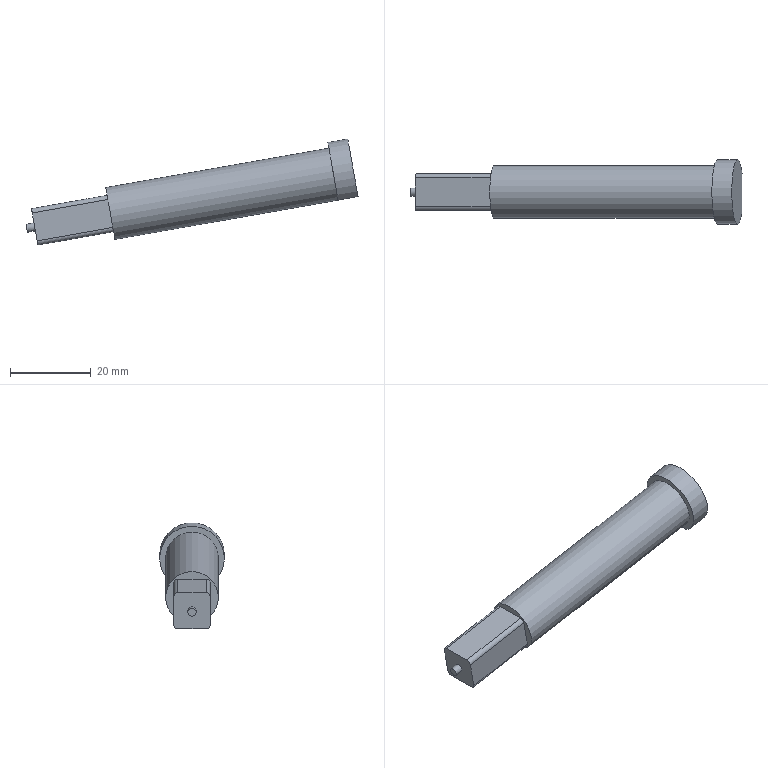Part | NX | features solid 2 | 1 solid | 17 faces | box 82.057 x 16 x 26.251 mm | volume 9952 mm3 | plane 10 | cylinder 7 | commonest cylinder face diameters 2.1 x4 2 x1 13 x1 16 x1